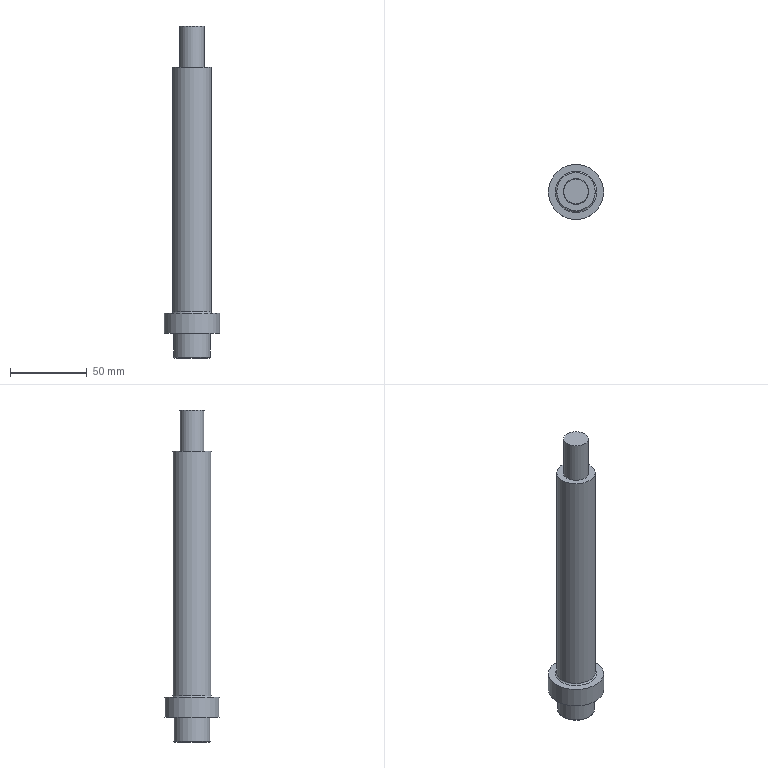Part | STEP file | 1_id1746_x_t | 1 solid | 29 faces | box 36 x 36 x 216 mm | volume 99455 mm3 | plane 18 | cylinder 6 | cone 4 | torus 1 | commonest cylinder face diameters 16.8 x2 16 x1 24 x1 25 x1 36 x1
STEP:
#1=CARTESIAN_POINT('',(825.935,385.,-17.5));
#2=VERTEX_POINT('',#1);
#3=CARTESIAN_POINT('',(839.435,385.,-17.5));
#4=DIRECTION('',(0.,0.,1.));
#5=DIRECTION('',(-1.,0.,0.));
#6=AXIS2_PLACEMENT_3D('',#3,#4,#5);
#7=CIRCLE('',#6,13.5);
#8=EDGE_CURVE('',#2,#2,#7,.T.);
#9=ORIENTED_EDGE('',*,*,#8,.T.);
#10=EDGE_LOOP('',(#9));
#11=FACE_BOUND('',#10,.T.);
#12=CARTESIAN_POINT('',(826.935,385.,-16.5));
#13=VERTEX_POINT('',#12);
#14=CARTESIAN_POINT('',(839.435,385.,-16.5));
#15=DIRECTION('',(0.,0.,-1.));
#16=DIRECTION('',(-1.,0.,0.));
#17=AXIS2_PLACEMENT_3D('',#14,#15,#16);
#18=CIRCLE('',#17,12.5);
#19=EDGE_CURVE('',#13,#13,#18,.T.);
#20=ORIENTED_EDGE('',*,*,#19,.T.);
#21=EDGE_LOOP('',(#20));
#22=FACE_BOUND('',#21,.T.);
#23=CARTESIAN_POINT('',(839.435,385.,-16.5));
#24=DIRECTION('',(0.,0.,-1.));
#25=DIRECTION('',(1.,0.,0.));
#26=AXIS2_PLACEMENT_3D('',#23,#24,#25);
#27=TOROIDAL_SURFACE('',#26,13.5,1.);
#28=ADVANCED_FACE('',(#11,#22),#27,.F.);
#29=CARTESIAN_POINT('',(857.435,385.,-30.5));
#30=VERTEX_POINT('',#29);
#31=CARTESIAN_POINT('',(839.435,385.,-30.5));
#32=DIRECTION('',(0.,0.,-1.));
#33=DIRECTION('',(1.,0.,0.));
#34=AXIS2_PLACEMENT_3D('',#31,#32,#33);
#35=CIRCLE('',#34,18.);
#36=EDGE_CURVE('',#30,#30,#35,.T.);
#37=ORIENTED_EDGE('',*,*,#36,.F.);
#38=EDGE_LOOP('',(#37));
#39=FACE_BOUND('',#38,.T.);
#40=CARTESIAN_POINT('',(857.435,385.,-17.5));
#41=VERTEX_POINT('',#40);
#42=CARTESIAN_POINT('',(839.435,385.,-17.5));
#43=DIRECTION('',(0.,0.,1.));
#44=DIRECTION('',(1.,0.,0.));
#45=AXIS2_PLACEMENT_3D('',#42,#43,#44);
#46=CIRCLE('',#45,18.);
#47=EDGE_CURVE('',#41,#41,#46,.T.);
#48=ORIENTED_EDGE('',*,*,#47,.F.);
#49=EDGE_LOOP('',(#48));
#50=FACE_BOUND('',#49,.T.);
#51=CARTESIAN_POINT('',(839.435,385.,-24.));
#52=DIRECTION('',(0.,0.,1.));
#53=DIRECTION('',(-1.,0.,0.));
#54=AXIS2_PLACEMENT_3D('',#51,#52,#53);
#55=CYLINDRICAL_SURFACE('',#54,18.);
#56=ADVANCED_FACE('',(#39,#50),#55,.T.);
#57=CARTESIAN_POINT('',(847.835,385.,142.5));
#58=VERTEX_POINT('',#57);
#59=CARTESIAN_POINT('',(847.835,385.,-30.5));
#60=VERTEX_POINT('',#59);
#61=CARTESIAN_POINT('',(847.835,385.,86.));
#62=DIRECTION('',(0.,0.,-1.));
#63=VECTOR('',#62,1.);
#64=LINE('',#61,#63);
#65=EDGE_CURVE('',#58,#60,#64,.T.);
#66=ORIENTED_EDGE('',*,*,#65,.F.);
#67=CARTESIAN_POINT('',(831.035,385.,142.5));
#68=VERTEX_POINT('',#67);
#69=CARTESIAN_POINT('',(839.435,385.,142.5));
#70=DIRECTION('',(0.,0.,-1.));
#71=DIRECTION('',(1.,0.,0.));
#72=AXIS2_PLACEMENT_3D('',#69,#70,#71);
#73=CIRCLE('',#72,8.4);
#74=EDGE_CURVE('',#68,#58,#73,.T.);
#75=ORIENTED_EDGE('',*,*,#74,.F.);
#76=CARTESIAN_POINT('',(831.035,385.,-30.5));
#77=VERTEX_POINT('',#76);
#78=CARTESIAN_POINT('',(831.035,385.,86.));
#79=DIRECTION('',(0.,0.,1.));
#80=VECTOR('',#79,1.);
#81=LINE('',#78,#80);
#82=EDGE_CURVE('',#77,#68,#81,.T.);
#83=ORIENTED_EDGE('',*,*,#82,.F.);
#84=CARTESIAN_POINT('',(839.435,385.,-30.5));
#85=DIRECTION('',(0.,0.,1.));
#86=DIRECTION('',(1.,0.,0.));
#87=AXIS2_PLACEMENT_3D('',#84,#85,#86);
#88=CIRCLE('',#87,8.4);
#89=EDGE_CURVE('',#60,#77,#88,.T.);
#90=ORIENTED_EDGE('',*,*,#89,.F.);
#91=EDGE_LOOP('',(#66,#75,#83,#90));
#92=FACE_OUTER_BOUND('',#91,.T.);
#93=CARTESIAN_POINT('',(839.435,385.,86.));
#94=DIRECTION('',(0.,0.,1.));
#95=DIRECTION('',(-1.,0.,0.));
#96=AXIS2_PLACEMENT_3D('',#93,#94,#95);
#97=CYLINDRICAL_SURFACE('',#96,8.4);
#98=ADVANCED_FACE('',(#92),#97,.F.);
#99=ORIENTED_EDGE('',*,*,#19,.F.);
#100=EDGE_LOOP('',(#99));
#101=FACE_BOUND('',#100,.T.);
#102=CARTESIAN_POINT('',(851.935,385.,142.5));
#103=VERTEX_POINT('',#102);
#104=CARTESIAN_POINT('',(839.435,385.,142.5));
#105=DIRECTION('',(0.,0.,1.));
#106=DIRECTION('',(1.,0.,0.));
#107=AXIS2_PLACEMENT_3D('',#104,#105,#106);
#108=CIRCLE('',#107,12.5);
#109=EDGE_CURVE('',#103,#103,#108,.T.);
#110=ORIENTED_EDGE('',*,*,#109,.F.);
#111=EDGE_LOOP('',(#110));
#112=FACE_BOUND('',#111,.T.);
#113=CARTESIAN_POINT('',(839.435,385.,92.5));
#114=DIRECTION('',(0.,0.,1.));
#115=DIRECTION('',(-1.,0.,0.));
#116=AXIS2_PLACEMENT_3D('',#113,#114,#115);
#117=CYLINDRICAL_SURFACE('',#116,12.5);
#118=ADVANCED_FACE('',(#101,#112),#117,.T.);
#119=CARTESIAN_POINT('',(847.435,385.,-30.5));
#120=VERTEX_POINT('',#119);
#121=CARTESIAN_POINT('',(839.435,385.,-30.5));
#122=DIRECTION('',(0.,0.,-1.));
#123=DIRECTION('',(1.,0.,0.));
#124=AXIS2_PLACEMENT_3D('',#121,#122,#123);
#125=CIRCLE('',#124,8.);
#126=EDGE_CURVE('',#120,#120,#125,.T.);
#127=ORIENTED_EDGE('',*,*,#126,.F.);
#128=EDGE_LOOP('',(#127));
#129=FACE_BOUND('',#128,.T.);
#130=CARTESIAN_POINT('',(847.435,385.,169.5));
#131=VERTEX_POINT('',#130);
#132=CARTESIAN_POINT('',(839.435,385.,169.5));
#133=DIRECTION('',(0.,0.,1.));
#134=DIRECTION('',(1.,0.,0.));
#135=AXIS2_PLACEMENT_3D('',#132,#133,#134);
#136=CIRCLE('',#135,8.);
#137=EDGE_CURVE('',#131,#131,#136,.T.);
#138=ORIENTED_EDGE('',*,*,#137,.F.);
#139=EDGE_LOOP('',(#138));
#140=FACE_BOUND('',#139,.T.);
#141=CARTESIAN_POINT('',(839.435,385.,99.5));
#142=DIRECTION('',(0.,0.,1.));
#143=DIRECTION('',(-1.,0.,0.));
#144=AXIS2_PLACEMENT_3D('',#141,#142,#143);
#145=CYLINDRICAL_SURFACE('',#144,8.);
#146=ADVANCED_FACE('',(#129,#140),#145,.T.);
#147=CARTESIAN_POINT('',(831.352,385.,-38.5));
#148=VERTEX_POINT('',#147);
#149=CARTESIAN_POINT('',(839.435,385.,-37.5));
#150=VERTEX_POINT('',#149);
#151=CARTESIAN_POINT('',(835.394,385.,-38.));
#152=DIRECTION('',(0.9924,0.,0.1228));
#153=VECTOR('',#152,1.);
#154=LINE('',#151,#153);
#155=EDGE_CURVE('',#148,#150,#154,.T.);
#156=ORIENTED_EDGE('',*,*,#155,.T.);
#157=CARTESIAN_POINT('',(847.518,385.,-38.5));
#158=VERTEX_POINT('',#157);
#159=CARTESIAN_POINT('',(843.477,385.,-38.));
#160=DIRECTION('',(0.9924,0.,-0.1228));
#161=VECTOR('',#160,1.);
#162=LINE('',#159,#161);
#163=EDGE_CURVE('',#150,#158,#162,.T.);
#164=ORIENTED_EDGE('',*,*,#163,.T.);
#165=CARTESIAN_POINT('',(846.435,380.958,-38.5));
#166=VERTEX_POINT('',#165);
#167=CARTESIAN_POINT('',(839.435,385.,-38.5));
#168=DIRECTION('',(0.,0.,-1.));
#169=DIRECTION('',(1.,0.,0.));
#170=AXIS2_PLACEMENT_3D('',#167,#168,#169);
#171=CIRCLE('',#170,8.083);
#172=EDGE_CURVE('',#158,#166,#171,.T.);
#173=ORIENTED_EDGE('',*,*,#172,.T.);
#174=CARTESIAN_POINT('',(839.435,376.917,-38.5));
#175=VERTEX_POINT('',#174);
#176=CARTESIAN_POINT('',(839.435,385.,-38.5));
#177=DIRECTION('',(0.,0.,-1.));
#178=DIRECTION('',(1.,0.,0.));
#179=AXIS2_PLACEMENT_3D('',#176,#177,#178);
#180=CIRCLE('',#179,8.083);
#181=EDGE_CURVE('',#166,#175,#180,.T.);
#182=ORIENTED_EDGE('',*,*,#181,.T.);
#183=CARTESIAN_POINT('',(832.435,380.958,-38.5));
#184=VERTEX_POINT('',#183);
#185=CARTESIAN_POINT('',(839.435,385.,-38.5));
#186=DIRECTION('',(0.,0.,-1.));
#187=DIRECTION('',(1.,0.,0.));
#188=AXIS2_PLACEMENT_3D('',#185,#186,#187);
#189=CIRCLE('',#188,8.083);
#190=EDGE_CURVE('',#175,#184,#189,.T.);
#191=ORIENTED_EDGE('',*,*,#190,.T.);
#192=CARTESIAN_POINT('',(839.435,385.,-38.5));
#193=DIRECTION('',(0.,0.,-1.));
#194=DIRECTION('',(1.,0.,0.));
#195=AXIS2_PLACEMENT_3D('',#192,#193,#194);
#196=CIRCLE('',#195,8.083);
#197=EDGE_CURVE('',#184,#148,#196,.T.);
#198=ORIENTED_EDGE('',*,*,#197,.T.);
#199=EDGE_LOOP('',(#156,#164,#173,#182,#191,#198));
#200=FACE_OUTER_BOUND('',#199,.T.);
#201=CARTESIAN_POINT('',(839.435,385.,-38.));
#202=DIRECTION('',(0.,0.,-1.));
#203=DIRECTION('',(-1.,0.,0.));
#204=AXIS2_PLACEMENT_3D('',#201,#202,#203);
#205=CONICAL_SURFACE('',#204,4.041,82.947);
#206=ADVANCED_FACE('',(#200),#205,.F.);
#207=CARTESIAN_POINT('',(851.435,385.,-46.));
#208=VERTEX_POINT('',#207);
#209=CARTESIAN_POINT('',(827.435,385.,-46.));
#210=VERTEX_POINT('',#209);
#211=CARTESIAN_POINT('',(839.435,385.,-46.));
#212=DIRECTION('',(0.,0.,-1.));
#213=DIRECTION('',(-1.,0.,0.));
#214=AXIS2_PLACEMENT_3D('',#211,#212,#213);
#215=CIRCLE('',#214,12.);
#216=EDGE_CURVE('',#208,#210,#215,.T.);
#217=ORIENTED_EDGE('',*,*,#216,.F.);
#218=CARTESIAN_POINT('',(839.435,385.,-46.));
#219=DIRECTION('',(0.,0.,-1.));
#220=DIRECTION('',(-1.,0.,0.));
#221=AXIS2_PLACEMENT_3D('',#218,#219,#220);
#222=CIRCLE('',#221,12.);
#223=EDGE_CURVE('',#210,#208,#222,.T.);
#224=ORIENTED_EDGE('',*,*,#223,.F.);
#225=EDGE_LOOP('',(#217,#224));
#226=FACE_BOUND('',#225,.T.);
#227=CARTESIAN_POINT('',(851.435,385.,-30.5));
#228=VERTEX_POINT('',#227);
#229=CARTESIAN_POINT('',(839.435,385.,-30.5));
#230=DIRECTION('',(0.,0.,1.));
#231=DIRECTION('',(1.,0.,0.));
#232=AXIS2_PLACEMENT_3D('',#229,#230,#231);
#233=CIRCLE('',#232,12.);
#234=EDGE_CURVE('',#228,#228,#233,.T.);
#235=ORIENTED_EDGE('',*,*,#234,.F.);
#236=EDGE_LOOP('',(#235));
#237=FACE_BOUND('',#236,.T.);
#238=CARTESIAN_POINT('',(839.435,385.,-38.5));
#239=DIRECTION('',(0.,0.,1.));
#240=DIRECTION('',(-1.,0.,0.));
#241=AXIS2_PLACEMENT_3D('',#238,#239,#240);
#242=CYLINDRICAL_SURFACE('',#241,12.);
#243=ADVANCED_FACE('',(#226,#237),#242,.T.);
#244=CARTESIAN_POINT('',(827.935,385.,-46.5));
#245=VERTEX_POINT('',#244);
#246=CARTESIAN_POINT('',(827.935,385.,-46.5));
#247=DIRECTION('',(0.7071,0.,-0.7071));
#248=VECTOR('',#247,1.);
#249=LINE('',#246,#248);
#250=EDGE_CURVE('',#210,#245,#249,.T.);
#251=ORIENTED_EDGE('',*,*,#250,.F.);
#252=ORIENTED_EDGE('',*,*,#223,.T.);
#253=CARTESIAN_POINT('',(850.935,385.,-46.5));
#254=VERTEX_POINT('',#253);
#255=CARTESIAN_POINT('',(850.935,385.,-46.5));
#256=DIRECTION('',(0.7071,0.,0.7071));
#257=VECTOR('',#256,1.);
#258=LINE('',#255,#257);
#259=EDGE_CURVE('',#254,#208,#258,.T.);
#260=ORIENTED_EDGE('',*,*,#259,.F.);
#261=CARTESIAN_POINT('',(839.435,385.,-46.5));
#262=DIRECTION('',(0.,0.,1.));
#263=DIRECTION('',(-1.,0.,0.));
#264=AXIS2_PLACEMENT_3D('',#261,#262,#263);
#265=CIRCLE('',#264,11.5);
#266=EDGE_CURVE('',#254,#245,#265,.T.);
#267=ORIENTED_EDGE('',*,*,#266,.T.);
#268=EDGE_LOOP('',(#251,#252,#260,#267));
#269=FACE_OUTER_BOUND('',#268,.T.);
#270=CARTESIAN_POINT('',(839.435,385.,-46.5));
#271=DIRECTION('',(0.,0.,1.));
#272=DIRECTION('',(1.,0.,0.));
#273=AXIS2_PLACEMENT_3D('',#270,#271,#272);
#274=CONICAL_SURFACE('',#273,11.5,45.);
#275=ADVANCED_FACE('',(#269),#274,.T.);
#276=ORIENTED_EDGE('',*,*,#126,.T.);
#277=EDGE_LOOP('',(#276));
#278=FACE_BOUND('',#277,.T.);
#279=ORIENTED_EDGE('',*,*,#89,.T.);
#280=CARTESIAN_POINT('',(839.435,385.,-30.5));
#281=DIRECTION('',(0.,0.,1.));
#282=DIRECTION('',(1.,0.,0.));
#283=AXIS2_PLACEMENT_3D('',#280,#281,#282);
#284=CIRCLE('',#283,8.4);
#285=EDGE_CURVE('',#77,#60,#284,.T.);
#286=ORIENTED_EDGE('',*,*,#285,.T.);
#287=EDGE_LOOP('',(#279,#286));
#288=FACE_BOUND('',#287,.T.);
#289=CARTESIAN_POINT('',(839.435,385.,-30.5));
#290=DIRECTION('',(0.,0.,1.));
#291=DIRECTION('',(-1.,0.,0.));
#292=AXIS2_PLACEMENT_3D('',#289,#290,#291);
#293=PLANE('',#292);
#294=ADVANCED_FACE('',(#278,#288),#293,.T.);
#295=ORIENTED_EDGE('',*,*,#250,.T.);
#296=CARTESIAN_POINT('',(839.435,385.,-46.5));
#297=DIRECTION('',(0.,0.,1.));
#298=DIRECTION('',(-1.,0.,0.));
#299=AXIS2_PLACEMENT_3D('',#296,#297,#298);
#300=CIRCLE('',#299,11.5);
#301=EDGE_CURVE('',#245,#254,#300,.T.);
#302=ORIENTED_EDGE('',*,*,#301,.T.);
#303=ORIENTED_EDGE('',*,*,#259,.T.);
#304=ORIENTED_EDGE('',*,*,#216,.T.);
#305=EDGE_LOOP('',(#295,#302,#303,#304));
#306=FACE_OUTER_BOUND('',#305,.T.);
#307=CARTESIAN_POINT('',(839.435,385.,-46.5));
#308=DIRECTION('',(0.,0.,1.));
#309=DIRECTION('',(1.,0.,0.));
#310=AXIS2_PLACEMENT_3D('',#307,#308,#309);
#311=CONICAL_SURFACE('',#310,11.5,45.);
#312=ADVANCED_FACE('',(#306),#311,.T.);
#313=CARTESIAN_POINT('',(839.435,376.917,-46.5));
#314=VERTEX_POINT('',#313);
#315=CARTESIAN_POINT('',(846.435,380.958,-46.5));
#316=VERTEX_POINT('',#315);
#317=CARTESIAN_POINT('',(842.935,378.938,-46.5));
#318=DIRECTION('',(0.866,0.5,0.));
#319=VECTOR('',#318,1.);
#320=LINE('',#317,#319);
#321=EDGE_CURVE('',#314,#316,#320,.T.);
#322=ORIENTED_EDGE('',*,*,#321,.T.);
#323=CARTESIAN_POINT('',(846.435,389.041,-46.5));
#324=VERTEX_POINT('',#323);
#325=CARTESIAN_POINT('',(846.435,385.,-46.5));
#326=DIRECTION('',(0.,1.,0.));
#327=VECTOR('',#326,1.);
#328=LINE('',#325,#327);
#329=EDGE_CURVE('',#316,#324,#328,.T.);
#330=ORIENTED_EDGE('',*,*,#329,.T.);
#331=CARTESIAN_POINT('',(839.435,393.083,-46.5));
#332=VERTEX_POINT('',#331);
#333=CARTESIAN_POINT('',(842.935,391.062,-46.5));
#334=DIRECTION('',(-0.866,0.5,0.));
#335=VECTOR('',#334,1.);
#336=LINE('',#333,#335);
#337=EDGE_CURVE('',#324,#332,#336,.T.);
#338=ORIENTED_EDGE('',*,*,#337,.T.);
#339=CARTESIAN_POINT('',(832.435,389.041,-46.5));
#340=VERTEX_POINT('',#339);
#341=CARTESIAN_POINT('',(835.935,391.062,-46.5));
#342=DIRECTION('',(-0.866,-0.5,0.));
#343=VECTOR('',#342,1.);
#344=LINE('',#341,#343);
#345=EDGE_CURVE('',#332,#340,#344,.T.);
#346=ORIENTED_EDGE('',*,*,#345,.T.);
#347=CARTESIAN_POINT('',(832.435,380.958,-46.5));
#348=VERTEX_POINT('',#347);
#349=CARTESIAN_POINT('',(832.435,385.,-46.5));
#350=DIRECTION('',(0.,-1.,0.));
#351=VECTOR('',#350,1.);
#352=LINE('',#349,#351);
#353=EDGE_CURVE('',#340,#348,#352,.T.);
#354=ORIENTED_EDGE('',*,*,#353,.T.);
#355=CARTESIAN_POINT('',(835.935,378.938,-46.5));
#356=DIRECTION('',(0.866,-0.5,0.));
#357=VECTOR('',#356,1.);
#358=LINE('',#355,#357);
#359=EDGE_CURVE('',#348,#314,#358,.T.);
#360=ORIENTED_EDGE('',*,*,#359,.T.);
#361=EDGE_LOOP('',(#322,#330,#338,#346,#354,#360));
#362=FACE_BOUND('',#361,.T.);
#363=ORIENTED_EDGE('',*,*,#266,.F.);
#364=ORIENTED_EDGE('',*,*,#301,.F.);
#365=EDGE_LOOP('',(#363,#364));
#366=FACE_BOUND('',#365,.T.);
#367=CARTESIAN_POINT('',(839.435,385.,-46.5));
#368=DIRECTION('',(0.,0.,-1.));
#369=DIRECTION('',(1.,0.,0.));
#370=AXIS2_PLACEMENT_3D('',#367,#368,#369);
#371=PLANE('',#370);
#372=ADVANCED_FACE('',(#362,#366),#371,.T.);
#373=CARTESIAN_POINT('',(842.935,378.938,-38.5));
#374=DIRECTION('',(0.866,0.5,0.));
#375=VECTOR('',#374,1.);
#376=LINE('',#373,#375);
#377=EDGE_CURVE('',#175,#166,#376,.T.);
#378=ORIENTED_EDGE('',*,*,#377,.F.);
#379=ORIENTED_EDGE('',*,*,#181,.F.);
#380=EDGE_LOOP('',(#378,#379));
#381=FACE_OUTER_BOUND('',#380,.T.);
#382=CARTESIAN_POINT('',(839.435,385.,-38.5));
#383=DIRECTION('',(0.,0.,-1.));
#384=DIRECTION('',(1.,0.,0.));
#385=AXIS2_PLACEMENT_3D('',#382,#383,#384);
#386=PLANE('',#385);
#387=ADVANCED_FACE('',(#381),#386,.F.);
#388=CARTESIAN_POINT('',(846.435,389.041,-38.5));
#389=VERTEX_POINT('',#388);
#390=CARTESIAN_POINT('',(846.435,385.,-38.5));
#391=DIRECTION('',(0.,1.,0.));
#392=VECTOR('',#391,1.);
#393=LINE('',#390,#392);
#394=EDGE_CURVE('',#166,#389,#393,.T.);
#395=ORIENTED_EDGE('',*,*,#394,.F.);
#396=ORIENTED_EDGE('',*,*,#172,.F.);
#397=CARTESIAN_POINT('',(839.435,385.,-38.5));
#398=DIRECTION('',(0.,0.,-1.));
#399=DIRECTION('',(1.,0.,0.));
#400=AXIS2_PLACEMENT_3D('',#397,#398,#399);
#401=CIRCLE('',#400,8.083);
#402=EDGE_CURVE('',#389,#158,#401,.T.);
#403=ORIENTED_EDGE('',*,*,#402,.F.);
#404=EDGE_LOOP('',(#395,#396,#403));
#405=FACE_OUTER_BOUND('',#404,.T.);
#406=CARTESIAN_POINT('',(839.435,385.,-38.5));
#407=DIRECTION('',(0.,0.,-1.));
#408=DIRECTION('',(1.,0.,0.));
#409=AXIS2_PLACEMENT_3D('',#406,#407,#408);
#410=PLANE('',#409);
#411=ADVANCED_FACE('',(#405),#410,.F.);
#412=CARTESIAN_POINT('',(839.435,393.083,-38.5));
#413=VERTEX_POINT('',#412);
#414=CARTESIAN_POINT('',(842.935,391.062,-38.5));
#415=DIRECTION('',(-0.866,0.5,0.));
#416=VECTOR('',#415,1.);
#417=LINE('',#414,#416);
#418=EDGE_CURVE('',#389,#413,#417,.T.);
#419=ORIENTED_EDGE('',*,*,#418,.F.);
#420=CARTESIAN_POINT('',(839.435,385.,-38.5));
#421=DIRECTION('',(0.,0.,-1.));
#422=DIRECTION('',(1.,0.,0.));
#423=AXIS2_PLACEMENT_3D('',#420,#421,#422);
#424=CIRCLE('',#423,8.083);
#425=EDGE_CURVE('',#413,#389,#424,.T.);
#426=ORIENTED_EDGE('',*,*,#425,.F.);
#427=EDGE_LOOP('',(#419,#426));
#428=FACE_OUTER_BOUND('',#427,.T.);
#429=CARTESIAN_POINT('',(839.435,385.,-38.5));
#430=DIRECTION('',(0.,0.,-1.));
#431=DIRECTION('',(1.,0.,0.));
#432=AXIS2_PLACEMENT_3D('',#429,#430,#431);
#433=PLANE('',#432);
#434=ADVANCED_FACE('',(#428),#433,.F.);
#435=CARTESIAN_POINT('',(832.435,389.041,-38.5));
#436=VERTEX_POINT('',#435);
#437=CARTESIAN_POINT('',(835.935,391.062,-38.5));
#438=DIRECTION('',(-0.866,-0.5,0.));
#439=VECTOR('',#438,1.);
#440=LINE('',#437,#439);
#441=EDGE_CURVE('',#413,#436,#440,.T.);
#442=ORIENTED_EDGE('',*,*,#441,.F.);
#443=CARTESIAN_POINT('',(839.435,385.,-38.5));
#444=DIRECTION('',(0.,0.,-1.));
#445=DIRECTION('',(1.,0.,0.));
#446=AXIS2_PLACEMENT_3D('',#443,#444,#445);
#447=CIRCLE('',#446,8.083);
#448=EDGE_CURVE('',#436,#413,#447,.T.);
#449=ORIENTED_EDGE('',*,*,#448,.F.);
#450=EDGE_LOOP('',(#442,#449));
#451=FACE_OUTER_BOUND('',#450,.T.);
#452=CARTESIAN_POINT('',(839.435,385.,-38.5));
#453=DIRECTION('',(0.,0.,-1.));
#454=DIRECTION('',(1.,0.,0.));
#455=AXIS2_PLACEMENT_3D('',#452,#453,#454);
#456=PLANE('',#455);
#457=ADVANCED_FACE('',(#451),#456,.F.);
#458=CARTESIAN_POINT('',(832.435,385.,-38.5));
#459=DIRECTION('',(0.,-1.,0.));
#460=VECTOR('',#459,1.);
#461=LINE('',#458,#460);
#462=EDGE_CURVE('',#436,#184,#461,.T.);
#463=ORIENTED_EDGE('',*,*,#462,.F.);
#464=CARTESIAN_POINT('',(839.435,385.,-38.5));
#465=DIRECTION('',(0.,0.,-1.));
#466=DIRECTION('',(1.,0.,0.));
#467=AXIS2_PLACEMENT_3D('',#464,#465,#466);
#468=CIRCLE('',#467,8.083);
#469=EDGE_CURVE('',#148,#436,#468,.T.);
#470=ORIENTED_EDGE('',*,*,#469,.F.);
#471=ORIENTED_EDGE('',*,*,#197,.F.);
#472=EDGE_LOOP('',(#463,#470,#471));
#473=FACE_OUTER_BOUND('',#472,.T.);
#474=CARTESIAN_POINT('',(839.435,385.,-38.5));
#475=DIRECTION('',(0.,0.,-1.));
#476=DIRECTION('',(1.,0.,0.));
#477=AXIS2_PLACEMENT_3D('',#474,#475,#476);
#478=PLANE('',#477);
#479=ADVANCED_FACE('',(#473),#478,.F.);
#480=CARTESIAN_POINT('',(835.935,378.938,-38.5));
#481=DIRECTION('',(0.866,-0.5,0.));
#482=VECTOR('',#481,1.);
#483=LINE('',#480,#482);
#484=EDGE_CURVE('',#184,#175,#483,.T.);
#485=ORIENTED_EDGE('',*,*,#484,.F.);
#486=ORIENTED_EDGE('',*,*,#190,.F.);
#487=EDGE_LOOP('',(#485,#486));
#488=FACE_OUTER_BOUND('',#487,.T.);
#489=CARTESIAN_POINT('',(839.435,385.,-38.5));
#490=DIRECTION('',(0.,0.,-1.));
#491=DIRECTION('',(1.,0.,0.));
#492=AXIS2_PLACEMENT_3D('',#489,#490,#491);
#493=PLANE('',#492);
#494=ADVANCED_FACE('',(#488),#493,.F.);
#495=ORIENTED_EDGE('',*,*,#155,.F.);
#496=ORIENTED_EDGE('',*,*,#469,.T.);
#497=ORIENTED_EDGE('',*,*,#448,.T.);
#498=ORIENTED_EDGE('',*,*,#425,.T.);
#499=ORIENTED_EDGE('',*,*,#402,.T.);
#500=ORIENTED_EDGE('',*,*,#163,.F.);
#501=EDGE_LOOP('',(#495,#496,#497,#498,#499,#500));
#502=FACE_OUTER_BOUND('',#501,.T.);
#503=CARTESIAN_POINT('',(839.435,385.,-38.));
#504=DIRECTION('',(0.,0.,-1.));
#505=DIRECTION('',(-1.,0.,0.));
#506=AXIS2_PLACEMENT_3D('',#503,#504,#505);
#507=CONICAL_SURFACE('',#506,4.041,82.947);
#508=ADVANCED_FACE('',(#502),#507,.F.);
#509=CARTESIAN_POINT('',(839.435,376.917,-42.5));
#510=DIRECTION('',(0.,0.,-1.));
#511=VECTOR('',#510,1.);
#512=LINE('',#509,#511);
#513=EDGE_CURVE('',#175,#314,#512,.T.);
#514=ORIENTED_EDGE('',*,*,#513,.F.);
#515=ORIENTED_EDGE('',*,*,#377,.T.);
#516=CARTESIAN_POINT('',(846.435,380.958,-42.5));
#517=DIRECTION('',(0.,0.,-1.));
#518=VECTOR('',#517,1.);
#519=LINE('',#516,#518);
#520=EDGE_CURVE('',#166,#316,#519,.T.);
#521=ORIENTED_EDGE('',*,*,#520,.T.);
#522=ORIENTED_EDGE('',*,*,#321,.F.);
#523=EDGE_LOOP('',(#514,#515,#521,#522));
#524=FACE_OUTER_BOUND('',#523,.T.);
#525=CARTESIAN_POINT('',(842.935,378.938,-42.5));
#526=DIRECTION('',(-0.5,0.866,0.));
#527=DIRECTION('',(0.,0.,-1.));
#528=AXIS2_PLACEMENT_3D('',#525,#526,#527);
#529=PLANE('',#528);
#530=ADVANCED_FACE('',(#524),#529,.T.);
#531=CARTESIAN_POINT('',(832.435,380.958,-42.5));
#532=DIRECTION('',(0.,0.,-1.));
#533=VECTOR('',#532,1.);
#534=LINE('',#531,#533);
#535=EDGE_CURVE('',#184,#348,#534,.T.);
#536=ORIENTED_EDGE('',*,*,#535,.F.);
#537=ORIENTED_EDGE('',*,*,#484,.T.);
#538=ORIENTED_EDGE('',*,*,#513,.T.);
#539=ORIENTED_EDGE('',*,*,#359,.F.);
#540=EDGE_LOOP('',(#536,#537,#538,#539));
#541=FACE_OUTER_BOUND('',#540,.T.);
#542=CARTESIAN_POINT('',(835.935,378.938,-42.5));
#543=DIRECTION('',(0.5,0.866,0.));
#544=DIRECTION('',(0.,0.,1.));
#545=AXIS2_PLACEMENT_3D('',#542,#543,#544);
#546=PLANE('',#545);
#547=ADVANCED_FACE('',(#541),#546,.T.);
#548=CARTESIAN_POINT('',(832.435,389.041,-42.5));
#549=DIRECTION('',(0.,0.,-1.));
#550=VECTOR('',#549,1.);
#551=LINE('',#548,#550);
#552=EDGE_CURVE('',#436,#340,#551,.T.);
#553=ORIENTED_EDGE('',*,*,#552,.F.);
#554=ORIENTED_EDGE('',*,*,#462,.T.);
#555=ORIENTED_EDGE('',*,*,#535,.T.);
#556=ORIENTED_EDGE('',*,*,#353,.F.);
#557=EDGE_LOOP('',(#553,#554,#555,#556));
#558=FACE_OUTER_BOUND('',#557,.T.);
#559=CARTESIAN_POINT('',(832.435,385.,-42.5));
#560=DIRECTION('',(1.,0.,0.));
#561=DIRECTION('',(0.,0.,1.));
#562=AXIS2_PLACEMENT_3D('',#559,#560,#561);
#563=PLANE('',#562);
#564=ADVANCED_FACE('',(#558),#563,.T.);
#565=CARTESIAN_POINT('',(839.435,393.083,-42.5));
#566=DIRECTION('',(0.,0.,-1.));
#567=VECTOR('',#566,1.);
#568=LINE('',#565,#567);
#569=EDGE_CURVE('',#413,#332,#568,.T.);
#570=ORIENTED_EDGE('',*,*,#569,.F.);
#571=ORIENTED_EDGE('',*,*,#441,.T.);
#572=ORIENTED_EDGE('',*,*,#552,.T.);
#573=ORIENTED_EDGE('',*,*,#345,.F.);
#574=EDGE_LOOP('',(#570,#571,#572,#573));
#575=FACE_OUTER_BOUND('',#574,.T.);
#576=CARTESIAN_POINT('',(835.935,391.062,-42.5));
#577=DIRECTION('',(0.5,-0.866,0.));
#578=DIRECTION('',(0.,0.,1.));
#579=AXIS2_PLACEMENT_3D('',#576,#577,#578);
#580=PLANE('',#579);
#581=ADVANCED_FACE('',(#575),#580,.T.);
#582=CARTESIAN_POINT('',(846.435,389.041,-42.5));
#583=DIRECTION('',(0.,0.,-1.));
#584=VECTOR('',#583,1.);
#585=LINE('',#582,#584);
#586=EDGE_CURVE('',#389,#324,#585,.T.);
#587=ORIENTED_EDGE('',*,*,#586,.F.);
#588=ORIENTED_EDGE('',*,*,#418,.T.);
#589=ORIENTED_EDGE('',*,*,#569,.T.);
#590=ORIENTED_EDGE('',*,*,#337,.F.);
#591=EDGE_LOOP('',(#587,#588,#589,#590));
#592=FACE_OUTER_BOUND('',#591,.T.);
#593=CARTESIAN_POINT('',(842.935,391.062,-42.5));
#594=DIRECTION('',(-0.5,-0.866,0.));
#595=DIRECTION('',(0.,0.,-1.));
#596=AXIS2_PLACEMENT_3D('',#593,#594,#595);
#597=PLANE('',#596);
#598=ADVANCED_FACE('',(#592),#597,.T.);
#599=ORIENTED_EDGE('',*,*,#520,.F.);
#600=ORIENTED_EDGE('',*,*,#394,.T.);
#601=ORIENTED_EDGE('',*,*,#586,.T.);
#602=ORIENTED_EDGE('',*,*,#329,.F.);
#603=EDGE_LOOP('',(#599,#600,#601,#602));
#604=FACE_OUTER_BOUND('',#603,.T.);
#605=CARTESIAN_POINT('',(846.435,385.,-42.5));
#606=DIRECTION('',(-1.,0.,0.));
#607=DIRECTION('',(0.,0.,-1.));
#608=AXIS2_PLACEMENT_3D('',#605,#606,#607);
#609=PLANE('',#608);
#610=ADVANCED_FACE('',(#604),#609,.T.);
#611=ORIENTED_EDGE('',*,*,#137,.T.);
#612=EDGE_LOOP('',(#611));
#613=FACE_OUTER_BOUND('',#612,.T.);
#614=CARTESIAN_POINT('',(839.435,385.,169.5));
#615=DIRECTION('',(0.,0.,1.));
#616=DIRECTION('',(-1.,0.,0.));
#617=AXIS2_PLACEMENT_3D('',#614,#615,#616);
#618=PLANE('',#617);
#619=ADVANCED_FACE('',(#613),#618,.T.);
#620=ORIENTED_EDGE('',*,*,#47,.T.);
#621=EDGE_LOOP('',(#620));
#622=FACE_BOUND('',#621,.T.);
#623=ORIENTED_EDGE('',*,*,#8,.F.);
#624=EDGE_LOOP('',(#623));
#625=FACE_BOUND('',#624,.T.);
#626=CARTESIAN_POINT('',(839.435,385.,-17.5));
#627=DIRECTION('',(0.,0.,1.));
#628=DIRECTION('',(-1.,0.,0.));
#629=AXIS2_PLACEMENT_3D('',#626,#627,#628);
#630=PLANE('',#629);
#631=ADVANCED_FACE('',(#622,#625),#630,.T.);
#632=ORIENTED_EDGE('',*,*,#65,.T.);
#633=ORIENTED_EDGE('',*,*,#285,.F.);
#634=ORIENTED_EDGE('',*,*,#82,.T.);
#635=CARTESIAN_POINT('',(839.435,385.,142.5));
#636=DIRECTION('',(0.,0.,-1.));
#637=DIRECTION('',(1.,0.,0.));
#638=AXIS2_PLACEMENT_3D('',#635,#636,#637);
#639=CIRCLE('',#638,8.4);
#640=EDGE_CURVE('',#58,#68,#639,.T.);
#641=ORIENTED_EDGE('',*,*,#640,.F.);
#642=EDGE_LOOP('',(#632,#633,#634,#641));
#643=FACE_OUTER_BOUND('',#642,.T.);
#644=CARTESIAN_POINT('',(839.435,385.,86.));
#645=DIRECTION('',(0.,0.,1.));
#646=DIRECTION('',(-1.,0.,0.));
#647=AXIS2_PLACEMENT_3D('',#644,#645,#646);
#648=CYLINDRICAL_SURFACE('',#647,8.4);
#649=ADVANCED_FACE('',(#643),#648,.F.);
#650=ORIENTED_EDGE('',*,*,#640,.T.);
#651=ORIENTED_EDGE('',*,*,#74,.T.);
#652=EDGE_LOOP('',(#650,#651));
#653=FACE_BOUND('',#652,.T.);
#654=ORIENTED_EDGE('',*,*,#109,.T.);
#655=EDGE_LOOP('',(#654));
#656=FACE_BOUND('',#655,.T.);
#657=CARTESIAN_POINT('',(839.435,385.,142.5));
#658=DIRECTION('',(0.,0.,1.));
#659=DIRECTION('',(-1.,0.,0.));
#660=AXIS2_PLACEMENT_3D('',#657,#658,#659);
#661=PLANE('',#660);
#662=ADVANCED_FACE('',(#653,#656),#661,.T.);
#663=ORIENTED_EDGE('',*,*,#234,.T.);
#664=EDGE_LOOP('',(#663));
#665=FACE_BOUND('',#664,.T.);
#666=ORIENTED_EDGE('',*,*,#36,.T.);
#667=EDGE_LOOP('',(#666));
#668=FACE_BOUND('',#667,.T.);
#669=CARTESIAN_POINT('',(839.435,385.,-30.5));
#670=DIRECTION('',(0.,0.,-1.));
#671=DIRECTION('',(1.,0.,0.));
#672=AXIS2_PLACEMENT_3D('',#669,#670,#671);
#673=PLANE('',#672);
#674=ADVANCED_FACE('',(#665,#668),#673,.T.);
#675=CLOSED_SHELL('',(#28,#56,#98,#118,#146,#206,#243,#275,#294,#312,#372,#387,#411,#434,#457,#479,#494,#508,#530,#547,#564,#581,#598,#610,#619,#631,#649,#662,#674));
#676=MANIFOLD_SOLID_BREP('',#675);
#677=(LENGTH_UNIT()NAMED_UNIT(*)SI_UNIT(.MILLI.,.METRE.));
#678=UNCERTAINTY_MEASURE_WITH_UNIT(LENGTH_MEASURE(0.00002),#677,'','');
#679=(NAMED_UNIT(*)PLANE_ANGLE_UNIT()SI_UNIT($,.RADIAN.));
#680=PLANE_ANGLE_MEASURE_WITH_UNIT(PLANE_ANGLE_MEASURE(0.01745),#679);
#681=DIMENSIONAL_EXPONENTS(0.,0.,0.,0.,0.,0.,0.);
#682=(CONVERSION_BASED_UNIT('DEGREE',#680)NAMED_UNIT(#681)PLANE_ANGLE_UNIT());
#683=(NAMED_UNIT(*)SI_UNIT($,.STERADIAN.)SOLID_ANGLE_UNIT());
#684=(GEOMETRIC_REPRESENTATION_CONTEXT(3)GLOBAL_UNCERTAINTY_ASSIGNED_CONTEXT((#678))GLOBAL_UNIT_ASSIGNED_CONTEXT((#677,#682,#683))REPRESENTATION_CONTEXT('',''));
#685=ADVANCED_BREP_SHAPE_REPRESENTATION('',(#676),#684);